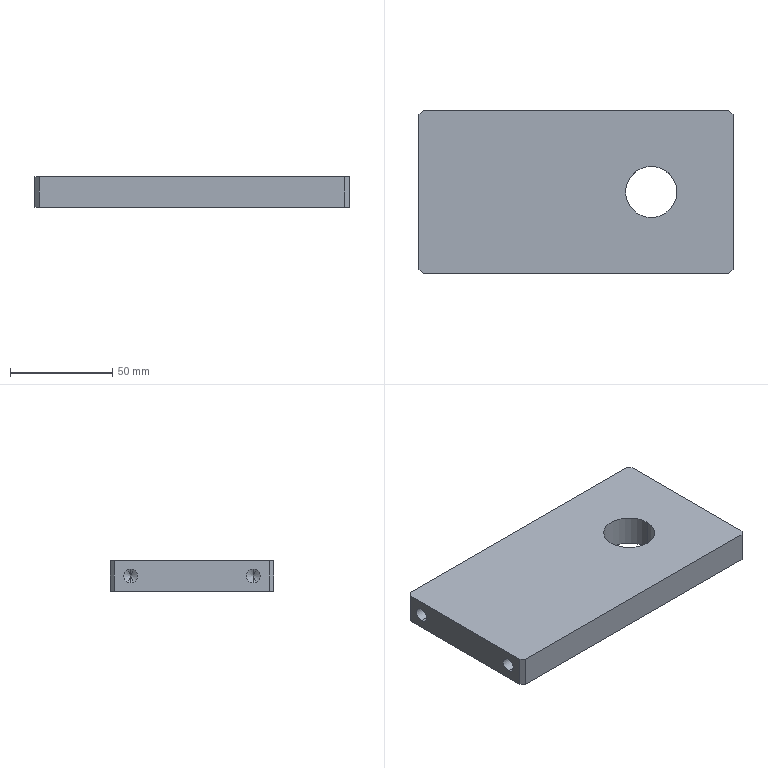Part | SolidWorks | features HoleWzd 2, Chamfer 1, Extrusion 1, MirrorPattern 1 | 1 solid | 28 faces | box 153.5 x 80 x 15 mm | volume 173749 mm3 | cylinder 10 | plane 10 | cone 8 | commonest cylinder face diameters 6.8 x8 25 x2
STEP:
#1=CARTESIAN_POINT('',(-57.,30.,-3.4));
#2=VERTEX_POINT('',#1);
#3=CARTESIAN_POINT('',(-57.,30.,3.4));
#4=VERTEX_POINT('',#3);
#5=CARTESIAN_POINT('',(-57.,30.,0.));
#6=DIRECTION('',(-1.,0.,0.));
#7=DIRECTION('',(0.,0.,1.));
#8=AXIS2_PLACEMENT_3D('',#5,#6,#7);
#9=CIRCLE('',#8,3.4);
#10=EDGE_CURVE('',#2,#4,#9,.T.);
#11=ORIENTED_EDGE('',*,*,#10,.F.);
#12=CARTESIAN_POINT('',(-76.75,30.,-3.4));
#13=VERTEX_POINT('',#12);
#14=CARTESIAN_POINT('',(-76.75,30.,-3.4));
#15=DIRECTION('',(-1.,0.,0.));
#16=VECTOR('',#15,1000.);
#17=LINE('',#14,#16);
#18=EDGE_CURVE('',#2,#13,#17,.T.);
#19=ORIENTED_EDGE('',*,*,#18,.T.);
#20=CARTESIAN_POINT('',(-76.75,30.,3.4));
#21=VERTEX_POINT('',#20);
#22=CARTESIAN_POINT('',(-76.75,30.,0.));
#23=DIRECTION('',(-1.,0.,0.));
#24=DIRECTION('',(0.,0.,1.));
#25=AXIS2_PLACEMENT_3D('',#22,#23,#24);
#26=CIRCLE('',#25,3.4);
#27=EDGE_CURVE('',#13,#21,#26,.T.);
#28=ORIENTED_EDGE('',*,*,#27,.T.);
#29=CARTESIAN_POINT('',(-76.75,30.,3.4));
#30=DIRECTION('',(-1.,0.,0.));
#31=VECTOR('',#30,1000.);
#32=LINE('',#29,#31);
#33=EDGE_CURVE('',#4,#21,#32,.T.);
#34=ORIENTED_EDGE('',*,*,#33,.F.);
#35=EDGE_LOOP('',(#11,#19,#28,#34));
#36=FACE_OUTER_BOUND('',#35,.T.);
#37=CARTESIAN_POINT('',(-76.75,30.,0.));
#38=DIRECTION('',(-1.,0.,0.));
#39=DIRECTION('',(0.,0.,1.));
#40=AXIS2_PLACEMENT_3D('',#37,#38,#39);
#41=CYLINDRICAL_SURFACE('',#40,3.4);
#42=ADVANCED_FACE('',(#36),#41,.F.);
#43=CARTESIAN_POINT('',(-54.957,30.,0.));
#44=VERTEX_POINT('',#43);
#45=CARTESIAN_POINT('',(-57.,30.,3.4));
#46=DIRECTION('',(-0.515,0.,0.8572));
#47=VECTOR('',#46,1000.);
#48=LINE('',#45,#47);
#49=EDGE_CURVE('',#44,#4,#48,.T.);
#50=ORIENTED_EDGE('',*,*,#49,.F.);
#51=CARTESIAN_POINT('',(-57.,30.,-3.4));
#52=DIRECTION('',(-0.515,0.,-0.8572));
#53=VECTOR('',#52,1000.);
#54=LINE('',#51,#53);
#55=EDGE_CURVE('',#44,#2,#54,.T.);
#56=ORIENTED_EDGE('',*,*,#55,.T.);
#57=ORIENTED_EDGE('',*,*,#10,.T.);
#58=EDGE_LOOP('',(#50,#56,#57));
#59=FACE_OUTER_BOUND('',#58,.T.);
#60=CARTESIAN_POINT('',(-57.,30.,0.));
#61=DIRECTION('',(-1.,0.,0.));
#62=DIRECTION('',(0.,0.,1.));
#63=AXIS2_PLACEMENT_3D('',#60,#61,#62);
#64=CONICAL_SURFACE('',#63,3.4,1.03);
#65=ADVANCED_FACE('',(#59),#64,.F.);
#66=CARTESIAN_POINT('',(-57.,-30.,-3.4));
#67=VERTEX_POINT('',#66);
#68=CARTESIAN_POINT('',(-57.,-30.,3.4));
#69=VERTEX_POINT('',#68);
#70=CARTESIAN_POINT('',(-57.,-30.,0.));
#71=DIRECTION('',(-1.,0.,0.));
#72=DIRECTION('',(0.,0.,1.));
#73=AXIS2_PLACEMENT_3D('',#70,#71,#72);
#74=CIRCLE('',#73,3.4);
#75=EDGE_CURVE('',#67,#69,#74,.T.);
#76=ORIENTED_EDGE('',*,*,#75,.F.);
#77=CARTESIAN_POINT('',(-76.75,-30.,-3.4));
#78=VERTEX_POINT('',#77);
#79=CARTESIAN_POINT('',(-76.75,-30.,-3.4));
#80=DIRECTION('',(-1.,0.,0.));
#81=VECTOR('',#80,1000.);
#82=LINE('',#79,#81);
#83=EDGE_CURVE('',#67,#78,#82,.T.);
#84=ORIENTED_EDGE('',*,*,#83,.T.);
#85=CARTESIAN_POINT('',(-76.75,-30.,3.4));
#86=VERTEX_POINT('',#85);
#87=CARTESIAN_POINT('',(-76.75,-30.,0.));
#88=DIRECTION('',(-1.,0.,0.));
#89=DIRECTION('',(0.,0.,1.));
#90=AXIS2_PLACEMENT_3D('',#87,#88,#89);
#91=CIRCLE('',#90,3.4);
#92=EDGE_CURVE('',#78,#86,#91,.T.);
#93=ORIENTED_EDGE('',*,*,#92,.T.);
#94=CARTESIAN_POINT('',(-76.75,-30.,3.4));
#95=DIRECTION('',(-1.,0.,0.));
#96=VECTOR('',#95,1000.);
#97=LINE('',#94,#96);
#98=EDGE_CURVE('',#69,#86,#97,.T.);
#99=ORIENTED_EDGE('',*,*,#98,.F.);
#100=EDGE_LOOP('',(#76,#84,#93,#99));
#101=FACE_OUTER_BOUND('',#100,.T.);
#102=CARTESIAN_POINT('',(-76.75,-30.,0.));
#103=DIRECTION('',(-1.,0.,0.));
#104=DIRECTION('',(0.,0.,1.));
#105=AXIS2_PLACEMENT_3D('',#102,#103,#104);
#106=CYLINDRICAL_SURFACE('',#105,3.4);
#107=ADVANCED_FACE('',(#101),#106,.F.);
#108=CARTESIAN_POINT('',(-54.957,-30.,0.));
#109=VERTEX_POINT('',#108);
#110=CARTESIAN_POINT('',(-57.,-30.,3.4));
#111=DIRECTION('',(-0.515,0.,0.8572));
#112=VECTOR('',#111,1000.);
#113=LINE('',#110,#112);
#114=EDGE_CURVE('',#109,#69,#113,.T.);
#115=ORIENTED_EDGE('',*,*,#114,.F.);
#116=CARTESIAN_POINT('',(-57.,-30.,-3.4));
#117=DIRECTION('',(-0.515,0.,-0.8572));
#118=VECTOR('',#117,1000.);
#119=LINE('',#116,#118);
#120=EDGE_CURVE('',#109,#67,#119,.T.);
#121=ORIENTED_EDGE('',*,*,#120,.T.);
#122=ORIENTED_EDGE('',*,*,#75,.T.);
#123=EDGE_LOOP('',(#115,#121,#122));
#124=FACE_OUTER_BOUND('',#123,.T.);
#125=CARTESIAN_POINT('',(-57.,-30.,0.));
#126=DIRECTION('',(-1.,0.,0.));
#127=DIRECTION('',(0.,0.,1.));
#128=AXIS2_PLACEMENT_3D('',#125,#126,#127);
#129=CONICAL_SURFACE('',#128,3.4,1.03);
#130=ADVANCED_FACE('',(#124),#129,.F.);
#131=CARTESIAN_POINT('',(57.,30.,3.4));
#132=VERTEX_POINT('',#131);
#133=CARTESIAN_POINT('',(57.,30.,-3.4));
#134=VERTEX_POINT('',#133);
#135=CARTESIAN_POINT('',(57.,30.,0.));
#136=DIRECTION('',(1.,0.,0.));
#137=DIRECTION('',(0.,0.,-1.));
#138=AXIS2_PLACEMENT_3D('',#135,#136,#137);
#139=CIRCLE('',#138,3.4);
#140=EDGE_CURVE('',#132,#134,#139,.T.);
#141=ORIENTED_EDGE('',*,*,#140,.F.);
#142=CARTESIAN_POINT('',(76.75,30.,3.4));
#143=VERTEX_POINT('',#142);
#144=CARTESIAN_POINT('',(76.75,30.,3.4));
#145=DIRECTION('',(1.,0.,0.));
#146=VECTOR('',#145,1000.);
#147=LINE('',#144,#146);
#148=EDGE_CURVE('',#132,#143,#147,.T.);
#149=ORIENTED_EDGE('',*,*,#148,.T.);
#150=CARTESIAN_POINT('',(76.75,30.,-3.4));
#151=VERTEX_POINT('',#150);
#152=CARTESIAN_POINT('',(76.75,30.,0.));
#153=DIRECTION('',(1.,0.,0.));
#154=DIRECTION('',(0.,0.,-1.));
#155=AXIS2_PLACEMENT_3D('',#152,#153,#154);
#156=CIRCLE('',#155,3.4);
#157=EDGE_CURVE('',#143,#151,#156,.T.);
#158=ORIENTED_EDGE('',*,*,#157,.T.);
#159=CARTESIAN_POINT('',(76.75,30.,-3.4));
#160=DIRECTION('',(1.,0.,0.));
#161=VECTOR('',#160,1000.);
#162=LINE('',#159,#161);
#163=EDGE_CURVE('',#134,#151,#162,.T.);
#164=ORIENTED_EDGE('',*,*,#163,.F.);
#165=EDGE_LOOP('',(#141,#149,#158,#164));
#166=FACE_OUTER_BOUND('',#165,.T.);
#167=CARTESIAN_POINT('',(76.75,30.,0.));
#168=DIRECTION('',(1.,0.,0.));
#169=DIRECTION('',(0.,0.,-1.));
#170=AXIS2_PLACEMENT_3D('',#167,#168,#169);
#171=CYLINDRICAL_SURFACE('',#170,3.4);
#172=ADVANCED_FACE('',(#166),#171,.F.);
#173=CARTESIAN_POINT('',(54.957,30.,0.));
#174=VERTEX_POINT('',#173);
#175=CARTESIAN_POINT('',(57.,30.,-3.4));
#176=DIRECTION('',(0.515,0.,-0.8572));
#177=VECTOR('',#176,1000.);
#178=LINE('',#175,#177);
#179=EDGE_CURVE('',#174,#134,#178,.T.);
#180=ORIENTED_EDGE('',*,*,#179,.F.);
#181=CARTESIAN_POINT('',(57.,30.,3.4));
#182=DIRECTION('',(0.515,0.,0.8572));
#183=VECTOR('',#182,1000.);
#184=LINE('',#181,#183);
#185=EDGE_CURVE('',#174,#132,#184,.T.);
#186=ORIENTED_EDGE('',*,*,#185,.T.);
#187=ORIENTED_EDGE('',*,*,#140,.T.);
#188=EDGE_LOOP('',(#180,#186,#187));
#189=FACE_OUTER_BOUND('',#188,.T.);
#190=CARTESIAN_POINT('',(57.,30.,0.));
#191=DIRECTION('',(1.,0.,0.));
#192=DIRECTION('',(0.,0.,-1.));
#193=AXIS2_PLACEMENT_3D('',#190,#191,#192);
#194=CONICAL_SURFACE('',#193,3.4,1.03);
#195=ADVANCED_FACE('',(#189),#194,.F.);
#196=CARTESIAN_POINT('',(57.,-30.,3.4));
#197=VERTEX_POINT('',#196);
#198=CARTESIAN_POINT('',(57.,-30.,-3.4));
#199=VERTEX_POINT('',#198);
#200=CARTESIAN_POINT('',(57.,-30.,0.));
#201=DIRECTION('',(1.,0.,0.));
#202=DIRECTION('',(0.,0.,-1.));
#203=AXIS2_PLACEMENT_3D('',#200,#201,#202);
#204=CIRCLE('',#203,3.4);
#205=EDGE_CURVE('',#197,#199,#204,.T.);
#206=ORIENTED_EDGE('',*,*,#205,.F.);
#207=CARTESIAN_POINT('',(76.75,-30.,3.4));
#208=VERTEX_POINT('',#207);
#209=CARTESIAN_POINT('',(76.75,-30.,3.4));
#210=DIRECTION('',(1.,0.,0.));
#211=VECTOR('',#210,1000.);
#212=LINE('',#209,#211);
#213=EDGE_CURVE('',#197,#208,#212,.T.);
#214=ORIENTED_EDGE('',*,*,#213,.T.);
#215=CARTESIAN_POINT('',(76.75,-30.,-3.4));
#216=VERTEX_POINT('',#215);
#217=CARTESIAN_POINT('',(76.75,-30.,0.));
#218=DIRECTION('',(1.,0.,0.));
#219=DIRECTION('',(0.,0.,-1.));
#220=AXIS2_PLACEMENT_3D('',#217,#218,#219);
#221=CIRCLE('',#220,3.4);
#222=EDGE_CURVE('',#208,#216,#221,.T.);
#223=ORIENTED_EDGE('',*,*,#222,.T.);
#224=CARTESIAN_POINT('',(76.75,-30.,-3.4));
#225=DIRECTION('',(1.,0.,0.));
#226=VECTOR('',#225,1000.);
#227=LINE('',#224,#226);
#228=EDGE_CURVE('',#199,#216,#227,.T.);
#229=ORIENTED_EDGE('',*,*,#228,.F.);
#230=EDGE_LOOP('',(#206,#214,#223,#229));
#231=FACE_OUTER_BOUND('',#230,.T.);
#232=CARTESIAN_POINT('',(76.75,-30.,0.));
#233=DIRECTION('',(1.,0.,0.));
#234=DIRECTION('',(0.,0.,-1.));
#235=AXIS2_PLACEMENT_3D('',#232,#233,#234);
#236=CYLINDRICAL_SURFACE('',#235,3.4);
#237=ADVANCED_FACE('',(#231),#236,.F.);
#238=CARTESIAN_POINT('',(54.957,-30.,0.));
#239=VERTEX_POINT('',#238);
#240=CARTESIAN_POINT('',(57.,-30.,-3.4));
#241=DIRECTION('',(0.515,0.,-0.8572));
#242=VECTOR('',#241,1000.);
#243=LINE('',#240,#242);
#244=EDGE_CURVE('',#239,#199,#243,.T.);
#245=ORIENTED_EDGE('',*,*,#244,.F.);
#246=CARTESIAN_POINT('',(57.,-30.,3.4));
#247=DIRECTION('',(0.515,0.,0.8572));
#248=VECTOR('',#247,1000.);
#249=LINE('',#246,#248);
#250=EDGE_CURVE('',#239,#197,#249,.T.);
#251=ORIENTED_EDGE('',*,*,#250,.T.);
#252=ORIENTED_EDGE('',*,*,#205,.T.);
#253=EDGE_LOOP('',(#245,#251,#252));
#254=FACE_OUTER_BOUND('',#253,.T.);
#255=CARTESIAN_POINT('',(57.,-30.,0.));
#256=DIRECTION('',(1.,0.,0.));
#257=DIRECTION('',(0.,0.,-1.));
#258=AXIS2_PLACEMENT_3D('',#255,#256,#257);
#259=CONICAL_SURFACE('',#258,3.4,1.03);
#260=ADVANCED_FACE('',(#254),#259,.F.);
#261=CARTESIAN_POINT('',(24.25,0.,-7.5));
#262=VERTEX_POINT('',#261);
#263=CARTESIAN_POINT('',(49.25,0.,-7.5));
#264=VERTEX_POINT('',#263);
#265=CARTESIAN_POINT('',(36.75,0.,-7.5));
#266=DIRECTION('',(0.,0.,1.));
#267=DIRECTION('',(1.,0.,0.));
#268=AXIS2_PLACEMENT_3D('',#265,#266,#267);
#269=CIRCLE('',#268,12.5);
#270=EDGE_CURVE('',#262,#264,#269,.T.);
#271=ORIENTED_EDGE('',*,*,#270,.F.);
#272=CARTESIAN_POINT('',(24.25,0.,7.5));
#273=VERTEX_POINT('',#272);
#274=CARTESIAN_POINT('',(24.25,0.,7.5));
#275=DIRECTION('',(0.,0.,1.));
#276=VECTOR('',#275,1000.);
#277=LINE('',#274,#276);
#278=EDGE_CURVE('',#262,#273,#277,.T.);
#279=ORIENTED_EDGE('',*,*,#278,.T.);
#280=CARTESIAN_POINT('',(49.25,0.,7.5));
#281=VERTEX_POINT('',#280);
#282=CARTESIAN_POINT('',(36.75,0.,7.5));
#283=DIRECTION('',(0.,0.,1.));
#284=DIRECTION('',(1.,0.,0.));
#285=AXIS2_PLACEMENT_3D('',#282,#283,#284);
#286=CIRCLE('',#285,12.5);
#287=EDGE_CURVE('',#273,#281,#286,.T.);
#288=ORIENTED_EDGE('',*,*,#287,.T.);
#289=CARTESIAN_POINT('',(49.25,0.,7.5));
#290=DIRECTION('',(0.,0.,1.));
#291=VECTOR('',#290,1000.);
#292=LINE('',#289,#291);
#293=EDGE_CURVE('',#264,#281,#292,.T.);
#294=ORIENTED_EDGE('',*,*,#293,.F.);
#295=EDGE_LOOP('',(#271,#279,#288,#294));
#296=FACE_OUTER_BOUND('',#295,.T.);
#297=CARTESIAN_POINT('',(36.75,0.,7.5));
#298=DIRECTION('',(0.,0.,1.));
#299=DIRECTION('',(1.,0.,0.));
#300=AXIS2_PLACEMENT_3D('',#297,#298,#299);
#301=CYLINDRICAL_SURFACE('',#300,12.5);
#302=ADVANCED_FACE('',(#296),#301,.F.);
#303=CARTESIAN_POINT('',(76.75,30.,0.));
#304=DIRECTION('',(1.,0.,0.));
#305=DIRECTION('',(0.,0.,-1.));
#306=AXIS2_PLACEMENT_3D('',#303,#304,#305);
#307=CIRCLE('',#306,3.4);
#308=EDGE_CURVE('',#151,#143,#307,.T.);
#309=ORIENTED_EDGE('',*,*,#308,.F.);
#310=ORIENTED_EDGE('',*,*,#157,.F.);
#311=EDGE_LOOP('',(#309,#310));
#312=FACE_BOUND('',#311,.T.);
#313=CARTESIAN_POINT('',(76.75,-30.,0.));
#314=DIRECTION('',(1.,0.,0.));
#315=DIRECTION('',(0.,0.,-1.));
#316=AXIS2_PLACEMENT_3D('',#313,#314,#315);
#317=CIRCLE('',#316,3.4);
#318=EDGE_CURVE('',#216,#208,#317,.T.);
#319=ORIENTED_EDGE('',*,*,#318,.F.);
#320=ORIENTED_EDGE('',*,*,#222,.F.);
#321=EDGE_LOOP('',(#319,#320));
#322=FACE_BOUND('',#321,.T.);
#323=CARTESIAN_POINT('',(76.75,-38.,7.5));
#324=VERTEX_POINT('',#323);
#325=CARTESIAN_POINT('',(76.75,38.,7.5));
#326=VERTEX_POINT('',#325);
#327=CARTESIAN_POINT('',(76.75,40.,7.5));
#328=DIRECTION('',(0.,1.,0.));
#329=VECTOR('',#328,1000.);
#330=LINE('',#327,#329);
#331=EDGE_CURVE('',#324,#326,#330,.T.);
#332=ORIENTED_EDGE('',*,*,#331,.F.);
#333=CARTESIAN_POINT('',(76.75,-38.,-7.5));
#334=VERTEX_POINT('',#333);
#335=CARTESIAN_POINT('',(76.75,-38.,7.5));
#336=DIRECTION('',(0.,0.,-1.));
#337=VECTOR('',#336,1000.);
#338=LINE('',#335,#337);
#339=EDGE_CURVE('',#324,#334,#338,.T.);
#340=ORIENTED_EDGE('',*,*,#339,.T.);
#341=CARTESIAN_POINT('',(76.75,38.,-7.5));
#342=VERTEX_POINT('',#341);
#343=CARTESIAN_POINT('',(76.75,40.,-7.5));
#344=DIRECTION('',(0.,1.,0.));
#345=VECTOR('',#344,1000.);
#346=LINE('',#343,#345);
#347=EDGE_CURVE('',#334,#342,#346,.T.);
#348=ORIENTED_EDGE('',*,*,#347,.T.);
#349=CARTESIAN_POINT('',(76.75,38.,7.5));
#350=DIRECTION('',(0.,0.,1.));
#351=VECTOR('',#350,1000.);
#352=LINE('',#349,#351);
#353=EDGE_CURVE('',#342,#326,#352,.T.);
#354=ORIENTED_EDGE('',*,*,#353,.T.);
#355=EDGE_LOOP('',(#332,#340,#348,#354));
#356=FACE_OUTER_BOUND('',#355,.T.);
#357=CARTESIAN_POINT('',(76.75,40.,7.5));
#358=DIRECTION('',(-1.,0.,0.));
#359=DIRECTION('',(0.,0.,1.));
#360=AXIS2_PLACEMENT_3D('',#357,#358,#359);
#361=PLANE('',#360);
#362=ADVANCED_FACE('',(#312,#322,#356),#361,.F.);
#363=CARTESIAN_POINT('',(74.75,40.,-7.5));
#364=VERTEX_POINT('',#363);
#365=CARTESIAN_POINT('',(-74.75,40.,-7.5));
#366=VERTEX_POINT('',#365);
#367=CARTESIAN_POINT('',(-76.75,40.,-7.5));
#368=DIRECTION('',(-1.,0.,0.));
#369=VECTOR('',#368,1000.);
#370=LINE('',#367,#369);
#371=EDGE_CURVE('',#364,#366,#370,.T.);
#372=ORIENTED_EDGE('',*,*,#371,.T.);
#373=CARTESIAN_POINT('',(-74.75,40.,7.5));
#374=VERTEX_POINT('',#373);
#375=CARTESIAN_POINT('',(-74.75,40.,7.5));
#376=DIRECTION('',(0.,0.,1.));
#377=VECTOR('',#376,1000.);
#378=LINE('',#375,#377);
#379=EDGE_CURVE('',#366,#374,#378,.T.);
#380=ORIENTED_EDGE('',*,*,#379,.T.);
#381=CARTESIAN_POINT('',(74.75,40.,7.5));
#382=VERTEX_POINT('',#381);
#383=CARTESIAN_POINT('',(-76.75,40.,7.5));
#384=DIRECTION('',(-1.,0.,0.));
#385=VECTOR('',#384,1000.);
#386=LINE('',#383,#385);
#387=EDGE_CURVE('',#382,#374,#386,.T.);
#388=ORIENTED_EDGE('',*,*,#387,.F.);
#389=CARTESIAN_POINT('',(74.75,40.,7.5));
#390=DIRECTION('',(0.,0.,-1.));
#391=VECTOR('',#390,1000.);
#392=LINE('',#389,#391);
#393=EDGE_CURVE('',#382,#364,#392,.T.);
#394=ORIENTED_EDGE('',*,*,#393,.T.);
#395=EDGE_LOOP('',(#372,#380,#388,#394));
#396=FACE_OUTER_BOUND('',#395,.T.);
#397=CARTESIAN_POINT('',(-76.75,40.,7.5));
#398=DIRECTION('',(0.,-1.,0.));
#399=DIRECTION('',(0.,0.,-1.));
#400=AXIS2_PLACEMENT_3D('',#397,#398,#399);
#401=PLANE('',#400);
#402=ADVANCED_FACE('',(#396),#401,.F.);
#403=CARTESIAN_POINT('',(-76.75,30.,0.));
#404=DIRECTION('',(-1.,0.,0.));
#405=DIRECTION('',(0.,0.,1.));
#406=AXIS2_PLACEMENT_3D('',#403,#404,#405);
#407=CIRCLE('',#406,3.4);
#408=EDGE_CURVE('',#21,#13,#407,.T.);
#409=ORIENTED_EDGE('',*,*,#408,.F.);
#410=ORIENTED_EDGE('',*,*,#27,.F.);
#411=EDGE_LOOP('',(#409,#410));
#412=FACE_BOUND('',#411,.T.);
#413=CARTESIAN_POINT('',(-76.75,-30.,0.));
#414=DIRECTION('',(-1.,0.,0.));
#415=DIRECTION('',(0.,0.,1.));
#416=AXIS2_PLACEMENT_3D('',#413,#414,#415);
#417=CIRCLE('',#416,3.4);
#418=EDGE_CURVE('',#86,#78,#417,.T.);
#419=ORIENTED_EDGE('',*,*,#418,.F.);
#420=ORIENTED_EDGE('',*,*,#92,.F.);
#421=EDGE_LOOP('',(#419,#420));
#422=FACE_BOUND('',#421,.T.);
#423=CARTESIAN_POINT('',(-76.75,38.,7.5));
#424=VERTEX_POINT('',#423);
#425=CARTESIAN_POINT('',(-76.75,-38.,7.5));
#426=VERTEX_POINT('',#425);
#427=CARTESIAN_POINT('',(-76.75,40.,7.5));
#428=DIRECTION('',(0.,-1.,0.));
#429=VECTOR('',#428,1000.);
#430=LINE('',#427,#429);
#431=EDGE_CURVE('',#424,#426,#430,.T.);
#432=ORIENTED_EDGE('',*,*,#431,.F.);
#433=CARTESIAN_POINT('',(-76.75,38.,-7.5));
#434=VERTEX_POINT('',#433);
#435=CARTESIAN_POINT('',(-76.75,38.,7.5));
#436=DIRECTION('',(0.,0.,-1.));
#437=VECTOR('',#436,1000.);
#438=LINE('',#435,#437);
#439=EDGE_CURVE('',#424,#434,#438,.T.);
#440=ORIENTED_EDGE('',*,*,#439,.T.);
#441=CARTESIAN_POINT('',(-76.75,-38.,-7.5));
#442=VERTEX_POINT('',#441);
#443=CARTESIAN_POINT('',(-76.75,40.,-7.5));
#444=DIRECTION('',(0.,-1.,0.));
#445=VECTOR('',#444,1000.);
#446=LINE('',#443,#445);
#447=EDGE_CURVE('',#434,#442,#446,.T.);
#448=ORIENTED_EDGE('',*,*,#447,.T.);
#449=CARTESIAN_POINT('',(-76.75,-38.,7.5));
#450=DIRECTION('',(0.,0.,1.));
#451=VECTOR('',#450,1000.);
#452=LINE('',#449,#451);
#453=EDGE_CURVE('',#442,#426,#452,.T.);
#454=ORIENTED_EDGE('',*,*,#453,.T.);
#455=EDGE_LOOP('',(#432,#440,#448,#454));
#456=FACE_OUTER_BOUND('',#455,.T.);
#457=CARTESIAN_POINT('',(-76.75,40.,7.5));
#458=DIRECTION('',(1.,0.,0.));
#459=DIRECTION('',(0.,0.,-1.));
#460=AXIS2_PLACEMENT_3D('',#457,#458,#459);
#461=PLANE('',#460);
#462=ADVANCED_FACE('',(#412,#422,#456),#461,.F.);
#463=CARTESIAN_POINT('',(-74.75,-40.,7.5));
#464=VERTEX_POINT('',#463);
#465=CARTESIAN_POINT('',(74.75,-40.,7.5));
#466=VERTEX_POINT('',#465);
#467=CARTESIAN_POINT('',(-76.75,-40.,7.5));
#468=DIRECTION('',(1.,0.,0.));
#469=VECTOR('',#468,1000.);
#470=LINE('',#467,#469);
#471=EDGE_CURVE('',#464,#466,#470,.T.);
#472=ORIENTED_EDGE('',*,*,#471,.F.);
#473=CARTESIAN_POINT('',(-74.75,-40.,-7.5));
#474=VERTEX_POINT('',#473);
#475=CARTESIAN_POINT('',(-74.75,-40.,7.5));
#476=DIRECTION('',(0.,0.,-1.));
#477=VECTOR('',#476,1000.);
#478=LINE('',#475,#477);
#479=EDGE_CURVE('',#464,#474,#478,.T.);
#480=ORIENTED_EDGE('',*,*,#479,.T.);
#481=CARTESIAN_POINT('',(74.75,-40.,-7.5));
#482=VERTEX_POINT('',#481);
#483=CARTESIAN_POINT('',(-76.75,-40.,-7.5));
#484=DIRECTION('',(1.,0.,0.));
#485=VECTOR('',#484,1000.);
#486=LINE('',#483,#485);
#487=EDGE_CURVE('',#474,#482,#486,.T.);
#488=ORIENTED_EDGE('',*,*,#487,.T.);
#489=CARTESIAN_POINT('',(74.75,-40.,7.5));
#490=DIRECTION('',(0.,0.,1.));
#491=VECTOR('',#490,1000.);
#492=LINE('',#489,#491);
#493=EDGE_CURVE('',#482,#466,#492,.T.);
#494=ORIENTED_EDGE('',*,*,#493,.T.);
#495=EDGE_LOOP('',(#472,#480,#488,#494));
#496=FACE_OUTER_BOUND('',#495,.T.);
#497=CARTESIAN_POINT('',(-76.75,-40.,7.5));
#498=DIRECTION('',(0.,1.,0.));
#499=DIRECTION('',(0.,0.,1.));
#500=AXIS2_PLACEMENT_3D('',#497,#498,#499);
#501=PLANE('',#500);
#502=ADVANCED_FACE('',(#496),#501,.F.);
#503=CARTESIAN_POINT('',(36.75,0.,7.5));
#504=DIRECTION('',(0.,0.,1.));
#505=DIRECTION('',(1.,0.,0.));
#506=AXIS2_PLACEMENT_3D('',#503,#504,#505);
#507=CIRCLE('',#506,12.5);
#508=EDGE_CURVE('',#281,#273,#507,.T.);
#509=ORIENTED_EDGE('',*,*,#508,.F.);
#510=ORIENTED_EDGE('',*,*,#287,.F.);
#511=EDGE_LOOP('',(#509,#510));
#512=FACE_BOUND('',#511,.T.);
#513=ORIENTED_EDGE('',*,*,#387,.T.);
#514=CARTESIAN_POINT('',(-57.375,57.375,7.5));
#515=DIRECTION('',(-0.7071,-0.7071,0.));
#516=VECTOR('',#515,1000.);
#517=LINE('',#514,#516);
#518=EDGE_CURVE('',#374,#424,#517,.T.);
#519=ORIENTED_EDGE('',*,*,#518,.T.);
#520=ORIENTED_EDGE('',*,*,#431,.T.);
#521=CARTESIAN_POINT('',(-57.375,-57.375,7.5));
#522=DIRECTION('',(0.7071,-0.7071,0.));
#523=VECTOR('',#522,1000.);
#524=LINE('',#521,#523);
#525=EDGE_CURVE('',#426,#464,#524,.T.);
#526=ORIENTED_EDGE('',*,*,#525,.T.);
#527=ORIENTED_EDGE('',*,*,#471,.T.);
#528=CARTESIAN_POINT('',(57.375,-57.375,7.5));
#529=DIRECTION('',(0.7071,0.7071,0.));
#530=VECTOR('',#529,1000.);
#531=LINE('',#528,#530);
#532=EDGE_CURVE('',#466,#324,#531,.T.);
#533=ORIENTED_EDGE('',*,*,#532,.T.);
#534=ORIENTED_EDGE('',*,*,#331,.T.);
#535=CARTESIAN_POINT('',(57.375,57.375,7.5));
#536=DIRECTION('',(-0.7071,0.7071,0.));
#537=VECTOR('',#536,1000.);
#538=LINE('',#535,#537);
#539=EDGE_CURVE('',#326,#382,#538,.T.);
#540=ORIENTED_EDGE('',*,*,#539,.T.);
#541=EDGE_LOOP('',(#513,#519,#520,#526,#527,#533,#534,#540));
#542=FACE_OUTER_BOUND('',#541,.T.);
#543=CARTESIAN_POINT('',(0.,0.,7.5));
#544=DIRECTION('',(0.,0.,1.));
#545=DIRECTION('',(1.,0.,0.));
#546=AXIS2_PLACEMENT_3D('',#543,#544,#545);
#547=PLANE('',#546);
#548=ADVANCED_FACE('',(#512,#542),#547,.T.);
#549=CARTESIAN_POINT('',(36.75,0.,-7.5));
#550=DIRECTION('',(0.,0.,1.));
#551=DIRECTION('',(1.,0.,0.));
#552=AXIS2_PLACEMENT_3D('',#549,#550,#551);
#553=CIRCLE('',#552,12.5);
#554=EDGE_CURVE('',#264,#262,#553,.T.);
#555=ORIENTED_EDGE('',*,*,#554,.T.);
#556=ORIENTED_EDGE('',*,*,#270,.T.);
#557=EDGE_LOOP('',(#555,#556));
#558=FACE_BOUND('',#557,.T.);
#559=ORIENTED_EDGE('',*,*,#447,.F.);
#560=CARTESIAN_POINT('',(-76.75,38.,-7.5));
#561=DIRECTION('',(0.7071,0.7071,0.));
#562=VECTOR('',#561,1000.);
#563=LINE('',#560,#562);
#564=EDGE_CURVE('',#434,#366,#563,.T.);
#565=ORIENTED_EDGE('',*,*,#564,.T.);
#566=ORIENTED_EDGE('',*,*,#371,.F.);
#567=CARTESIAN_POINT('',(74.75,40.,-7.5));
#568=DIRECTION('',(0.7071,-0.7071,0.));
#569=VECTOR('',#568,1000.);
#570=LINE('',#567,#569);
#571=EDGE_CURVE('',#364,#342,#570,.T.);
#572=ORIENTED_EDGE('',*,*,#571,.T.);
#573=ORIENTED_EDGE('',*,*,#347,.F.);
#574=CARTESIAN_POINT('',(76.75,-38.,-7.5));
#575=DIRECTION('',(-0.7071,-0.7071,0.));
#576=VECTOR('',#575,1000.);
#577=LINE('',#574,#576);
#578=EDGE_CURVE('',#334,#482,#577,.T.);
#579=ORIENTED_EDGE('',*,*,#578,.T.);
#580=ORIENTED_EDGE('',*,*,#487,.F.);
#581=CARTESIAN_POINT('',(-74.75,-40.,-7.5));
#582=DIRECTION('',(-0.7071,0.7071,0.));
#583=VECTOR('',#582,1000.);
#584=LINE('',#581,#583);
#585=EDGE_CURVE('',#474,#442,#584,.T.);
#586=ORIENTED_EDGE('',*,*,#585,.T.);
#587=EDGE_LOOP('',(#559,#565,#566,#572,#573,#579,#580,#586));
#588=FACE_OUTER_BOUND('',#587,.T.);
#589=CARTESIAN_POINT('',(0.,0.,-7.5));
#590=DIRECTION('',(0.,0.,1.));
#591=DIRECTION('',(1.,0.,0.));
#592=AXIS2_PLACEMENT_3D('',#589,#590,#591);
#593=PLANE('',#592);
#594=ADVANCED_FACE('',(#558,#588),#593,.F.);
#595=ORIENTED_EDGE('',*,*,#278,.F.);
#596=ORIENTED_EDGE('',*,*,#554,.F.);
#597=ORIENTED_EDGE('',*,*,#293,.T.);
#598=ORIENTED_EDGE('',*,*,#508,.T.);
#599=EDGE_LOOP('',(#595,#596,#597,#598));
#600=FACE_OUTER_BOUND('',#599,.T.);
#601=CARTESIAN_POINT('',(36.75,0.,7.5));
#602=DIRECTION('',(0.,0.,1.));
#603=DIRECTION('',(1.,0.,0.));
#604=AXIS2_PLACEMENT_3D('',#601,#602,#603);
#605=CYLINDRICAL_SURFACE('',#604,12.5);
#606=ADVANCED_FACE('',(#600),#605,.F.);
#607=ORIENTED_EDGE('',*,*,#250,.F.);
#608=ORIENTED_EDGE('',*,*,#244,.T.);
#609=CARTESIAN_POINT('',(57.,-30.,0.));
#610=DIRECTION('',(1.,0.,0.));
#611=DIRECTION('',(0.,0.,-1.));
#612=AXIS2_PLACEMENT_3D('',#609,#610,#611);
#613=CIRCLE('',#612,3.4);
#614=EDGE_CURVE('',#199,#197,#613,.T.);
#615=ORIENTED_EDGE('',*,*,#614,.T.);
#616=EDGE_LOOP('',(#607,#608,#615));
#617=FACE_OUTER_BOUND('',#616,.T.);
#618=CARTESIAN_POINT('',(57.,-30.,0.));
#619=DIRECTION('',(1.,0.,0.));
#620=DIRECTION('',(0.,0.,-1.));
#621=AXIS2_PLACEMENT_3D('',#618,#619,#620);
#622=CONICAL_SURFACE('',#621,3.4,1.03);
#623=ADVANCED_FACE('',(#617),#622,.F.);
#624=ORIENTED_EDGE('',*,*,#213,.F.);
#625=ORIENTED_EDGE('',*,*,#614,.F.);
#626=ORIENTED_EDGE('',*,*,#228,.T.);
#627=ORIENTED_EDGE('',*,*,#318,.T.);
#628=EDGE_LOOP('',(#624,#625,#626,#627));
#629=FACE_OUTER_BOUND('',#628,.T.);
#630=CARTESIAN_POINT('',(76.75,-30.,0.));
#631=DIRECTION('',(1.,0.,0.));
#632=DIRECTION('',(0.,0.,-1.));
#633=AXIS2_PLACEMENT_3D('',#630,#631,#632);
#634=CYLINDRICAL_SURFACE('',#633,3.4);
#635=ADVANCED_FACE('',(#629),#634,.F.);
#636=ORIENTED_EDGE('',*,*,#185,.F.);
#637=ORIENTED_EDGE('',*,*,#179,.T.);
#638=CARTESIAN_POINT('',(57.,30.,0.));
#639=DIRECTION('',(1.,0.,0.));
#640=DIRECTION('',(0.,0.,-1.));
#641=AXIS2_PLACEMENT_3D('',#638,#639,#640);
#642=CIRCLE('',#641,3.4);
#643=EDGE_CURVE('',#134,#132,#642,.T.);
#644=ORIENTED_EDGE('',*,*,#643,.T.);
#645=EDGE_LOOP('',(#636,#637,#644));
#646=FACE_OUTER_BOUND('',#645,.T.);
#647=CARTESIAN_POINT('',(57.,30.,0.));
#648=DIRECTION('',(1.,0.,0.));
#649=DIRECTION('',(0.,0.,-1.));
#650=AXIS2_PLACEMENT_3D('',#647,#648,#649);
#651=CONICAL_SURFACE('',#650,3.4,1.03);
#652=ADVANCED_FACE('',(#646),#651,.F.);
#653=ORIENTED_EDGE('',*,*,#148,.F.);
#654=ORIENTED_EDGE('',*,*,#643,.F.);
#655=ORIENTED_EDGE('',*,*,#163,.T.);
#656=ORIENTED_EDGE('',*,*,#308,.T.);
#657=EDGE_LOOP('',(#653,#654,#655,#656));
#658=FACE_OUTER_BOUND('',#657,.T.);
#659=CARTESIAN_POINT('',(76.75,30.,0.));
#660=DIRECTION('',(1.,0.,0.));
#661=DIRECTION('',(0.,0.,-1.));
#662=AXIS2_PLACEMENT_3D('',#659,#660,#661);
#663=CYLINDRICAL_SURFACE('',#662,3.4);
#664=ADVANCED_FACE('',(#658),#663,.F.);
#665=ORIENTED_EDGE('',*,*,#120,.F.);
#666=ORIENTED_EDGE('',*,*,#114,.T.);
#667=CARTESIAN_POINT('',(-57.,-30.,0.));
#668=DIRECTION('',(-1.,0.,0.));
#669=DIRECTION('',(0.,0.,1.));
#670=AXIS2_PLACEMENT_3D('',#667,#668,#669);
#671=CIRCLE('',#670,3.4);
#672=EDGE_CURVE('',#69,#67,#671,.T.);
#673=ORIENTED_EDGE('',*,*,#672,.T.);
#674=EDGE_LOOP('',(#665,#666,#673));
#675=FACE_OUTER_BOUND('',#674,.T.);
#676=CARTESIAN_POINT('',(-57.,-30.,0.));
#677=DIRECTION('',(-1.,0.,0.));
#678=DIRECTION('',(0.,0.,1.));
#679=AXIS2_PLACEMENT_3D('',#676,#677,#678);
#680=CONICAL_SURFACE('',#679,3.4,1.03);
#681=ADVANCED_FACE('',(#675),#680,.F.);
#682=ORIENTED_EDGE('',*,*,#83,.F.);
#683=ORIENTED_EDGE('',*,*,#672,.F.);
#684=ORIENTED_EDGE('',*,*,#98,.T.);
#685=ORIENTED_EDGE('',*,*,#418,.T.);
#686=EDGE_LOOP('',(#682,#683,#684,#685));
#687=FACE_OUTER_BOUND('',#686,.T.);
#688=CARTESIAN_POINT('',(-76.75,-30.,0.));
#689=DIRECTION('',(-1.,0.,0.));
#690=DIRECTION('',(0.,0.,1.));
#691=AXIS2_PLACEMENT_3D('',#688,#689,#690);
#692=CYLINDRICAL_SURFACE('',#691,3.4);
#693=ADVANCED_FACE('',(#687),#692,.F.);
#694=ORIENTED_EDGE('',*,*,#55,.F.);
#695=ORIENTED_EDGE('',*,*,#49,.T.);
#696=CARTESIAN_POINT('',(-57.,30.,0.));
#697=DIRECTION('',(-1.,0.,0.));
#698=DIRECTION('',(0.,0.,1.));
#699=AXIS2_PLACEMENT_3D('',#696,#697,#698);
#700=CIRCLE('',#699,3.4);
#701=EDGE_CURVE('',#4,#2,#700,.T.);
#702=ORIENTED_EDGE('',*,*,#701,.T.);
#703=EDGE_LOOP('',(#694,#695,#702));
#704=FACE_OUTER_BOUND('',#703,.T.);
#705=CARTESIAN_POINT('',(-57.,30.,0.));
#706=DIRECTION('',(-1.,0.,0.));
#707=DIRECTION('',(0.,0.,1.));
#708=AXIS2_PLACEMENT_3D('',#705,#706,#707);
#709=CONICAL_SURFACE('',#708,3.4,1.03);
#710=ADVANCED_FACE('',(#704),#709,.F.);
#711=ORIENTED_EDGE('',*,*,#18,.F.);
#712=ORIENTED_EDGE('',*,*,#701,.F.);
#713=ORIENTED_EDGE('',*,*,#33,.T.);
#714=ORIENTED_EDGE('',*,*,#408,.T.);
#715=EDGE_LOOP('',(#711,#712,#713,#714));
#716=FACE_OUTER_BOUND('',#715,.T.);
#717=CARTESIAN_POINT('',(-76.75,30.,0.));
#718=DIRECTION('',(-1.,0.,0.));
#719=DIRECTION('',(0.,0.,1.));
#720=AXIS2_PLACEMENT_3D('',#717,#718,#719);
#721=CYLINDRICAL_SURFACE('',#720,3.4);
#722=ADVANCED_FACE('',(#716),#721,.F.);
#723=ORIENTED_EDGE('',*,*,#518,.F.);
#724=ORIENTED_EDGE('',*,*,#379,.F.);
#725=ORIENTED_EDGE('',*,*,#564,.F.);
#726=ORIENTED_EDGE('',*,*,#439,.F.);
#727=EDGE_LOOP('',(#723,#724,#725,#726));
#728=FACE_OUTER_BOUND('',#727,.T.);
#729=CARTESIAN_POINT('',(-76.75,38.,7.5));
#730=DIRECTION('',(0.7071,-0.7071,0.));
#731=DIRECTION('',(0.,0.,-1.));
#732=AXIS2_PLACEMENT_3D('',#729,#730,#731);
#733=PLANE('',#732);
#734=ADVANCED_FACE('',(#728),#733,.F.);
#735=ORIENTED_EDGE('',*,*,#525,.F.);
#736=ORIENTED_EDGE('',*,*,#453,.F.);
#737=ORIENTED_EDGE('',*,*,#585,.F.);
#738=ORIENTED_EDGE('',*,*,#479,.F.);
#739=EDGE_LOOP('',(#735,#736,#737,#738));
#740=FACE_OUTER_BOUND('',#739,.T.);
#741=CARTESIAN_POINT('',(-74.75,-40.,7.5));
#742=DIRECTION('',(0.7071,0.7071,0.));
#743=DIRECTION('',(0.,0.,-1.));
#744=AXIS2_PLACEMENT_3D('',#741,#742,#743);
#745=PLANE('',#744);
#746=ADVANCED_FACE('',(#740),#745,.F.);
#747=ORIENTED_EDGE('',*,*,#532,.F.);
#748=ORIENTED_EDGE('',*,*,#493,.F.);
#749=ORIENTED_EDGE('',*,*,#578,.F.);
#750=ORIENTED_EDGE('',*,*,#339,.F.);
#751=EDGE_LOOP('',(#747,#748,#749,#750));
#752=FACE_OUTER_BOUND('',#751,.T.);
#753=CARTESIAN_POINT('',(76.75,-38.,7.5));
#754=DIRECTION('',(-0.7071,0.7071,0.));
#755=DIRECTION('',(0.,0.,-1.));
#756=AXIS2_PLACEMENT_3D('',#753,#754,#755);
#757=PLANE('',#756);
#758=ADVANCED_FACE('',(#752),#757,.F.);
#759=ORIENTED_EDGE('',*,*,#539,.F.);
#760=ORIENTED_EDGE('',*,*,#353,.F.);
#761=ORIENTED_EDGE('',*,*,#571,.F.);
#762=ORIENTED_EDGE('',*,*,#393,.F.);
#763=EDGE_LOOP('',(#759,#760,#761,#762));
#764=FACE_OUTER_BOUND('',#763,.T.);
#765=CARTESIAN_POINT('',(74.75,40.,7.5));
#766=DIRECTION('',(-0.7071,-0.7071,0.));
#767=DIRECTION('',(0.,0.,-1.));
#768=AXIS2_PLACEMENT_3D('',#765,#766,#767);
#769=PLANE('',#768);
#770=ADVANCED_FACE('',(#764),#769,.F.);
#771=CLOSED_SHELL('',(#42,#65,#107,#130,#172,#195,#237,#260,#302,#362,#402,#462,#502,#548,#594,#606,#623,#635,#652,#664,#681,#693,#710,#722,#734,#746,#758,#770));
#772=MANIFOLD_SOLID_BREP('',#771);
#773=CARTESIAN_POINT('',(0.,0.,0.));
#774=DIRECTION('',(0.,0.,1.));
#775=DIRECTION('',(1.,0.,0.));
#776=AXIS2_PLACEMENT_3D('',#773,#774,#775);
#777=(LENGTH_UNIT()NAMED_UNIT(*)SI_UNIT(.MILLI.,.METRE.));
#778=UNCERTAINTY_MEASURE_WITH_UNIT(LENGTH_MEASURE(0.00001),#777,'','');
#779=(NAMED_UNIT(*)PLANE_ANGLE_UNIT()SI_UNIT($,.RADIAN.));
#780=(NAMED_UNIT(*)SI_UNIT($,.STERADIAN.)SOLID_ANGLE_UNIT());
#781=(GEOMETRIC_REPRESENTATION_CONTEXT(3)GLOBAL_UNCERTAINTY_ASSIGNED_CONTEXT((#778))GLOBAL_UNIT_ASSIGNED_CONTEXT((#777,#779,#780))REPRESENTATION_CONTEXT('',''));
#782=ADVANCED_BREP_SHAPE_REPRESENTATION('',(#772,#776),#781);